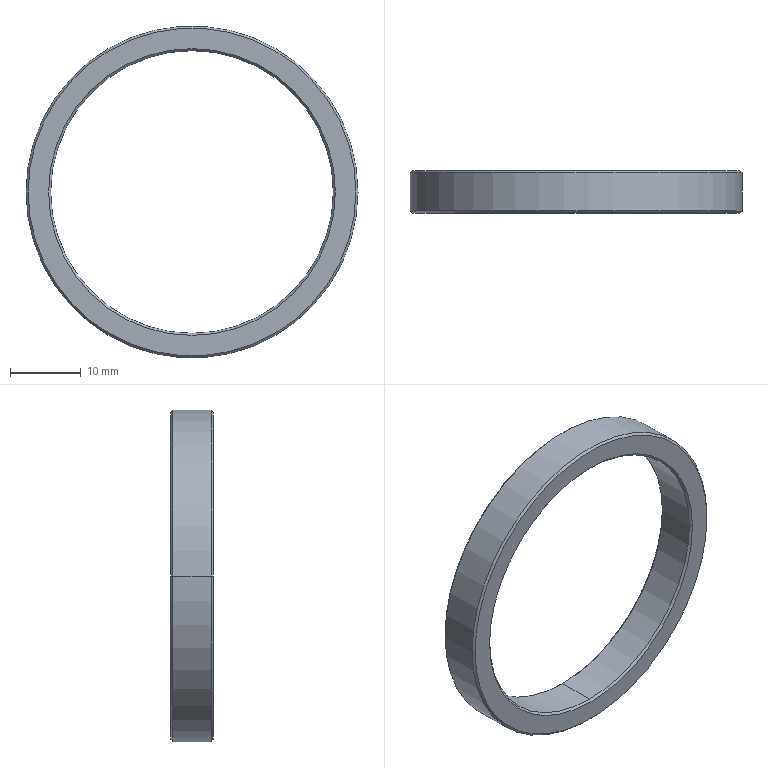Part | NX | 1 solid | 14 faces | box 47 x 6 x 47 mm | volume 2845 mm3 | cone 8 | cylinder 4 | plane 2 | commonest cylinder face diameters 40 x2 47 x2
STEP:
#1=CARTESIAN_POINT('',(23.2,0.,0.));
#2=VERTEX_POINT('',#1);
#3=CARTESIAN_POINT('',(-23.2,0.,0.));
#4=VERTEX_POINT('',#3);
#5=CARTESIAN_POINT('',(0.,0.,0.));
#6=DIRECTION('',(0.,1.,0.));
#7=DIRECTION('',(1.,0.,0.));
#8=AXIS2_PLACEMENT_3D('',#5,#6,#7);
#9=CIRCLE('',#8,23.2);
#10=EDGE_CURVE('',#2,#4,#9,.T.);
#11=ORIENTED_EDGE('',*,*,#10,.F.);
#12=CARTESIAN_POINT('',(0.,0.,0.));
#13=DIRECTION('',(0.,1.,0.));
#14=DIRECTION('',(1.,0.,0.));
#15=AXIS2_PLACEMENT_3D('',#12,#13,#14);
#16=CIRCLE('',#15,23.2);
#17=EDGE_CURVE('',#4,#2,#16,.T.);
#18=ORIENTED_EDGE('',*,*,#17,.F.);
#19=EDGE_LOOP('',(#11,#18));
#20=FACE_BOUND('',#19,.T.);
#21=CARTESIAN_POINT('',(20.3,0.,0.));
#22=VERTEX_POINT('',#21);
#23=CARTESIAN_POINT('',(-20.3,0.,0.));
#24=VERTEX_POINT('',#23);
#25=CARTESIAN_POINT('',(0.,0.,0.));
#26=DIRECTION('',(0.,-1.,0.));
#27=DIRECTION('',(-1.,0.,0.));
#28=AXIS2_PLACEMENT_3D('',#25,#26,#27);
#29=CIRCLE('',#28,20.3);
#30=EDGE_CURVE('',#22,#24,#29,.T.);
#31=ORIENTED_EDGE('',*,*,#30,.F.);
#32=CARTESIAN_POINT('',(0.,0.,0.));
#33=DIRECTION('',(0.,-1.,0.));
#34=DIRECTION('',(-1.,0.,0.));
#35=AXIS2_PLACEMENT_3D('',#32,#33,#34);
#36=CIRCLE('',#35,20.3);
#37=EDGE_CURVE('',#24,#22,#36,.T.);
#38=ORIENTED_EDGE('',*,*,#37,.F.);
#39=EDGE_LOOP('',(#31,#38));
#40=FACE_BOUND('',#39,.T.);
#41=CARTESIAN_POINT('',(0.,0.,0.));
#42=DIRECTION('',(0.,1.,0.));
#43=DIRECTION('',(1.,0.,0.));
#44=AXIS2_PLACEMENT_3D('',#41,#42,#43);
#45=PLANE('',#44);
#46=ADVANCED_FACE('',(#20,#40),#45,.F.);
#47=CARTESIAN_POINT('',(23.5,5.7,0.));
#48=VERTEX_POINT('',#47);
#49=CARTESIAN_POINT('',(-23.5,5.7,0.));
#50=VERTEX_POINT('',#49);
#51=CARTESIAN_POINT('',(0.,5.7,0.));
#52=DIRECTION('',(0.,-1.,0.));
#53=DIRECTION('',(-1.,0.,0.));
#54=AXIS2_PLACEMENT_3D('',#51,#52,#53);
#55=CIRCLE('',#54,23.5);
#56=EDGE_CURVE('',#48,#50,#55,.T.);
#57=ORIENTED_EDGE('',*,*,#56,.T.);
#58=CARTESIAN_POINT('',(-23.5,0.3,0.));
#59=VERTEX_POINT('',#58);
#60=CARTESIAN_POINT('',(-23.5,0.,0.));
#61=DIRECTION('',(0.,1.,0.));
#62=VECTOR('',#61,1000.);
#63=LINE('',#60,#62);
#64=EDGE_CURVE('',#50,#59,#63,.F.);
#65=ORIENTED_EDGE('',*,*,#64,.T.);
#66=CARTESIAN_POINT('',(23.5,0.3,0.));
#67=VERTEX_POINT('',#66);
#68=CARTESIAN_POINT('',(0.,0.3,0.));
#69=DIRECTION('',(0.,1.,0.));
#70=DIRECTION('',(1.,0.,0.));
#71=AXIS2_PLACEMENT_3D('',#68,#69,#70);
#72=CIRCLE('',#71,23.5);
#73=EDGE_CURVE('',#59,#67,#72,.T.);
#74=ORIENTED_EDGE('',*,*,#73,.T.);
#75=CARTESIAN_POINT('',(23.5,0.,0.));
#76=DIRECTION('',(0.,1.,0.));
#77=VECTOR('',#76,1000.);
#78=LINE('',#75,#77);
#79=EDGE_CURVE('',#48,#67,#78,.F.);
#80=ORIENTED_EDGE('',*,*,#79,.F.);
#81=EDGE_LOOP('',(#57,#65,#74,#80));
#82=FACE_BOUND('',#81,.T.);
#83=CARTESIAN_POINT('',(0.,0.,0.));
#84=DIRECTION('',(0.,1.,0.));
#85=DIRECTION('',(1.,0.,0.));
#86=AXIS2_PLACEMENT_3D('',#83,#84,#85);
#87=CYLINDRICAL_SURFACE('',#86,23.5);
#88=ADVANCED_FACE('',(#82),#87,.T.);
#89=CARTESIAN_POINT('',(0.,5.7,-20.));
#90=VERTEX_POINT('',#89);
#91=CARTESIAN_POINT('',(-20.,5.7,0.));
#92=VERTEX_POINT('',#91);
#93=CARTESIAN_POINT('',(0.,5.7,0.));
#94=DIRECTION('',(0.,1.,0.));
#95=DIRECTION('',(1.,0.,0.));
#96=AXIS2_PLACEMENT_3D('',#93,#94,#95);
#97=CIRCLE('',#96,20.);
#98=EDGE_CURVE('',#90,#92,#97,.T.);
#99=ORIENTED_EDGE('',*,*,#98,.T.);
#100=CARTESIAN_POINT('',(0.,5.7,20.));
#101=VERTEX_POINT('',#100);
#102=CARTESIAN_POINT('',(0.,5.7,0.));
#103=DIRECTION('',(0.,1.,0.));
#104=DIRECTION('',(1.,0.,0.));
#105=AXIS2_PLACEMENT_3D('',#102,#103,#104);
#106=CIRCLE('',#105,20.);
#107=EDGE_CURVE('',#92,#101,#106,.T.);
#108=ORIENTED_EDGE('',*,*,#107,.T.);
#109=CARTESIAN_POINT('',(0.,0.3,20.));
#110=VERTEX_POINT('',#109);
#111=CARTESIAN_POINT('',(0.,6.,20.));
#112=DIRECTION('',(0.,1.,0.));
#113=VECTOR('',#112,1000.);
#114=LINE('',#111,#113);
#115=EDGE_CURVE('',#110,#101,#114,.T.);
#116=ORIENTED_EDGE('',*,*,#115,.F.);
#117=CARTESIAN_POINT('',(-20.,0.3,0.));
#118=VERTEX_POINT('',#117);
#119=CARTESIAN_POINT('',(0.,0.3,0.));
#120=DIRECTION('',(0.,-1.,0.));
#121=DIRECTION('',(-1.,0.,0.));
#122=AXIS2_PLACEMENT_3D('',#119,#120,#121);
#123=CIRCLE('',#122,20.);
#124=EDGE_CURVE('',#110,#118,#123,.T.);
#125=ORIENTED_EDGE('',*,*,#124,.T.);
#126=CARTESIAN_POINT('',(0.,0.3,-20.));
#127=VERTEX_POINT('',#126);
#128=CARTESIAN_POINT('',(0.,0.3,0.));
#129=DIRECTION('',(0.,-1.,0.));
#130=DIRECTION('',(-1.,0.,0.));
#131=AXIS2_PLACEMENT_3D('',#128,#129,#130);
#132=CIRCLE('',#131,20.);
#133=EDGE_CURVE('',#118,#127,#132,.T.);
#134=ORIENTED_EDGE('',*,*,#133,.T.);
#135=CARTESIAN_POINT('',(0.,6.,-20.));
#136=DIRECTION('',(0.,1.,0.));
#137=VECTOR('',#136,1000.);
#138=LINE('',#135,#137);
#139=EDGE_CURVE('',#127,#90,#138,.T.);
#140=ORIENTED_EDGE('',*,*,#139,.T.);
#141=EDGE_LOOP('',(#99,#108,#116,#125,#134,#140));
#142=FACE_BOUND('',#141,.T.);
#143=CARTESIAN_POINT('',(0.,6.,0.));
#144=DIRECTION('',(0.,1.,0.));
#145=DIRECTION('',(0.,0.,-1.));
#146=AXIS2_PLACEMENT_3D('',#143,#144,#145);
#147=CYLINDRICAL_SURFACE('',#146,20.);
#148=ADVANCED_FACE('',(#142),#147,.F.);
#149=CARTESIAN_POINT('',(23.2,6.,0.));
#150=VERTEX_POINT('',#149);
#151=CARTESIAN_POINT('',(-23.2,6.,0.));
#152=VERTEX_POINT('',#151);
#153=CARTESIAN_POINT('',(0.,6.,0.));
#154=DIRECTION('',(0.,-1.,0.));
#155=DIRECTION('',(-1.,0.,0.));
#156=AXIS2_PLACEMENT_3D('',#153,#154,#155);
#157=CIRCLE('',#156,23.2);
#158=EDGE_CURVE('',#150,#152,#157,.T.);
#159=ORIENTED_EDGE('',*,*,#158,.F.);
#160=CARTESIAN_POINT('',(0.,6.,0.));
#161=DIRECTION('',(0.,-1.,0.));
#162=DIRECTION('',(-1.,0.,0.));
#163=AXIS2_PLACEMENT_3D('',#160,#161,#162);
#164=CIRCLE('',#163,23.2);
#165=EDGE_CURVE('',#152,#150,#164,.T.);
#166=ORIENTED_EDGE('',*,*,#165,.F.);
#167=EDGE_LOOP('',(#159,#166));
#168=FACE_BOUND('',#167,.T.);
#169=CARTESIAN_POINT('',(20.3,6.,0.));
#170=VERTEX_POINT('',#169);
#171=CARTESIAN_POINT('',(-20.3,6.,0.));
#172=VERTEX_POINT('',#171);
#173=CARTESIAN_POINT('',(0.,6.,0.));
#174=DIRECTION('',(0.,1.,0.));
#175=DIRECTION('',(1.,0.,0.));
#176=AXIS2_PLACEMENT_3D('',#173,#174,#175);
#177=CIRCLE('',#176,20.3);
#178=EDGE_CURVE('',#170,#172,#177,.T.);
#179=ORIENTED_EDGE('',*,*,#178,.F.);
#180=CARTESIAN_POINT('',(0.,6.,0.));
#181=DIRECTION('',(0.,1.,0.));
#182=DIRECTION('',(1.,0.,0.));
#183=AXIS2_PLACEMENT_3D('',#180,#181,#182);
#184=CIRCLE('',#183,20.3);
#185=EDGE_CURVE('',#172,#170,#184,.T.);
#186=ORIENTED_EDGE('',*,*,#185,.F.);
#187=EDGE_LOOP('',(#179,#186));
#188=FACE_BOUND('',#187,.T.);
#189=CARTESIAN_POINT('',(0.,6.,0.));
#190=DIRECTION('',(0.,1.,0.));
#191=DIRECTION('',(1.,0.,0.));
#192=AXIS2_PLACEMENT_3D('',#189,#190,#191);
#193=PLANE('',#192);
#194=ADVANCED_FACE('',(#168,#188),#193,.T.);
#195=CARTESIAN_POINT('',(0.,0.3,0.));
#196=DIRECTION('',(0.,1.,0.));
#197=DIRECTION('',(1.,0.,0.));
#198=AXIS2_PLACEMENT_3D('',#195,#196,#197);
#199=CIRCLE('',#198,23.5);
#200=EDGE_CURVE('',#67,#59,#199,.T.);
#201=ORIENTED_EDGE('',*,*,#200,.F.);
#202=CARTESIAN_POINT('',(23.2,0.,0.));
#203=DIRECTION('',(0.7071,0.7071,0.));
#204=VECTOR('',#203,1000.);
#205=LINE('',#202,#204);
#206=EDGE_CURVE('',#2,#67,#205,.T.);
#207=ORIENTED_EDGE('',*,*,#206,.F.);
#208=ORIENTED_EDGE('',*,*,#10,.T.);
#209=CARTESIAN_POINT('',(-23.2,0.,0.));
#210=DIRECTION('',(-0.7071,0.7071,0.));
#211=VECTOR('',#210,1000.);
#212=LINE('',#209,#211);
#213=EDGE_CURVE('',#4,#59,#212,.T.);
#214=ORIENTED_EDGE('',*,*,#213,.T.);
#215=EDGE_LOOP('',(#201,#207,#208,#214));
#216=FACE_BOUND('',#215,.T.);
#217=CARTESIAN_POINT('',(0.,0.,0.));
#218=DIRECTION('',(0.,1.,0.));
#219=DIRECTION('',(1.,0.,0.));
#220=AXIS2_PLACEMENT_3D('',#217,#218,#219);
#221=CONICAL_SURFACE('',#220,23.2,0.7854);
#222=ADVANCED_FACE('',(#216),#221,.T.);
#223=ORIENTED_EDGE('',*,*,#30,.T.);
#224=CARTESIAN_POINT('',(-20.3,0.,0.));
#225=DIRECTION('',(-0.7071,-0.7071,0.));
#226=VECTOR('',#225,1000.);
#227=LINE('',#224,#226);
#228=EDGE_CURVE('',#24,#118,#227,.F.);
#229=ORIENTED_EDGE('',*,*,#228,.T.);
#230=ORIENTED_EDGE('',*,*,#124,.F.);
#231=CARTESIAN_POINT('',(20.,0.3,0.));
#232=VERTEX_POINT('',#231);
#233=CARTESIAN_POINT('',(0.,0.3,0.));
#234=DIRECTION('',(0.,-1.,0.));
#235=DIRECTION('',(-1.,0.,0.));
#236=AXIS2_PLACEMENT_3D('',#233,#234,#235);
#237=CIRCLE('',#236,20.);
#238=EDGE_CURVE('',#232,#110,#237,.T.);
#239=ORIENTED_EDGE('',*,*,#238,.F.);
#240=CARTESIAN_POINT('',(20.3,0.,0.));
#241=DIRECTION('',(0.7071,-0.7071,0.));
#242=VECTOR('',#241,1000.);
#243=LINE('',#240,#242);
#244=EDGE_CURVE('',#22,#232,#243,.F.);
#245=ORIENTED_EDGE('',*,*,#244,.F.);
#246=EDGE_LOOP('',(#223,#229,#230,#239,#245));
#247=FACE_BOUND('',#246,.T.);
#248=CARTESIAN_POINT('',(0.,0.,0.));
#249=DIRECTION('',(0.,-1.,0.));
#250=DIRECTION('',(-1.,0.,0.));
#251=AXIS2_PLACEMENT_3D('',#248,#249,#250);
#252=CONICAL_SURFACE('',#251,20.3,0.7854);
#253=ADVANCED_FACE('',(#247),#252,.F.);
#254=ORIENTED_EDGE('',*,*,#158,.T.);
#255=CARTESIAN_POINT('',(-23.5,5.7,0.));
#256=DIRECTION('',(-0.7071,-0.7071,0.));
#257=VECTOR('',#256,1000.);
#258=LINE('',#255,#257);
#259=EDGE_CURVE('',#50,#152,#258,.F.);
#260=ORIENTED_EDGE('',*,*,#259,.F.);
#261=ORIENTED_EDGE('',*,*,#56,.F.);
#262=CARTESIAN_POINT('',(23.5,5.7,0.));
#263=DIRECTION('',(0.7071,-0.7071,0.));
#264=VECTOR('',#263,1000.);
#265=LINE('',#262,#264);
#266=EDGE_CURVE('',#48,#150,#265,.F.);
#267=ORIENTED_EDGE('',*,*,#266,.T.);
#268=EDGE_LOOP('',(#254,#260,#261,#267));
#269=FACE_BOUND('',#268,.T.);
#270=CARTESIAN_POINT('',(0.,5.7,0.));
#271=DIRECTION('',(0.,-1.,0.));
#272=DIRECTION('',(-1.,0.,0.));
#273=AXIS2_PLACEMENT_3D('',#270,#271,#272);
#274=CONICAL_SURFACE('',#273,23.5,0.7854);
#275=ADVANCED_FACE('',(#269),#274,.T.);
#276=ORIENTED_EDGE('',*,*,#98,.F.);
#277=CARTESIAN_POINT('',(20.,5.7,0.));
#278=VERTEX_POINT('',#277);
#279=CARTESIAN_POINT('',(0.,5.7,0.));
#280=DIRECTION('',(0.,1.,0.));
#281=DIRECTION('',(1.,0.,0.));
#282=AXIS2_PLACEMENT_3D('',#279,#280,#281);
#283=CIRCLE('',#282,20.);
#284=EDGE_CURVE('',#278,#90,#283,.T.);
#285=ORIENTED_EDGE('',*,*,#284,.F.);
#286=CARTESIAN_POINT('',(20.3,6.,0.));
#287=DIRECTION('',(0.7071,0.7071,0.));
#288=VECTOR('',#287,1000.);
#289=LINE('',#286,#288);
#290=EDGE_CURVE('',#278,#170,#289,.T.);
#291=ORIENTED_EDGE('',*,*,#290,.T.);
#292=ORIENTED_EDGE('',*,*,#178,.T.);
#293=CARTESIAN_POINT('',(-20.3,6.,0.));
#294=DIRECTION('',(-0.7071,0.7071,0.));
#295=VECTOR('',#294,1000.);
#296=LINE('',#293,#295);
#297=EDGE_CURVE('',#92,#172,#296,.T.);
#298=ORIENTED_EDGE('',*,*,#297,.F.);
#299=EDGE_LOOP('',(#276,#285,#291,#292,#298));
#300=FACE_BOUND('',#299,.T.);
#301=CARTESIAN_POINT('',(0.,6.,0.));
#302=DIRECTION('',(0.,1.,0.));
#303=DIRECTION('',(1.,0.,0.));
#304=AXIS2_PLACEMENT_3D('',#301,#302,#303);
#305=CONICAL_SURFACE('',#304,20.3,0.7854);
#306=ADVANCED_FACE('',(#300),#305,.F.);
#307=CARTESIAN_POINT('',(0.,0.3,0.));
#308=DIRECTION('',(0.,-1.,0.));
#309=DIRECTION('',(-1.,0.,0.));
#310=AXIS2_PLACEMENT_3D('',#307,#308,#309);
#311=CIRCLE('',#310,20.);
#312=EDGE_CURVE('',#127,#232,#311,.T.);
#313=ORIENTED_EDGE('',*,*,#312,.T.);
#314=ORIENTED_EDGE('',*,*,#238,.T.);
#315=ORIENTED_EDGE('',*,*,#115,.T.);
#316=CARTESIAN_POINT('',(0.,5.7,0.));
#317=DIRECTION('',(0.,1.,0.));
#318=DIRECTION('',(1.,0.,0.));
#319=AXIS2_PLACEMENT_3D('',#316,#317,#318);
#320=CIRCLE('',#319,20.);
#321=EDGE_CURVE('',#101,#278,#320,.T.);
#322=ORIENTED_EDGE('',*,*,#321,.T.);
#323=ORIENTED_EDGE('',*,*,#284,.T.);
#324=ORIENTED_EDGE('',*,*,#139,.F.);
#325=EDGE_LOOP('',(#313,#314,#315,#322,#323,#324));
#326=FACE_BOUND('',#325,.T.);
#327=CARTESIAN_POINT('',(0.,6.,0.));
#328=DIRECTION('',(0.,1.,0.));
#329=DIRECTION('',(0.,0.,-1.));
#330=AXIS2_PLACEMENT_3D('',#327,#328,#329);
#331=CYLINDRICAL_SURFACE('',#330,20.);
#332=ADVANCED_FACE('',(#326),#331,.F.);
#333=ORIENTED_EDGE('',*,*,#290,.F.);
#334=ORIENTED_EDGE('',*,*,#321,.F.);
#335=ORIENTED_EDGE('',*,*,#107,.F.);
#336=ORIENTED_EDGE('',*,*,#297,.T.);
#337=ORIENTED_EDGE('',*,*,#185,.T.);
#338=EDGE_LOOP('',(#333,#334,#335,#336,#337));
#339=FACE_BOUND('',#338,.T.);
#340=CARTESIAN_POINT('',(0.,6.,0.));
#341=DIRECTION('',(0.,1.,0.));
#342=DIRECTION('',(1.,0.,0.));
#343=AXIS2_PLACEMENT_3D('',#340,#341,#342);
#344=CONICAL_SURFACE('',#343,20.3,0.7854);
#345=ADVANCED_FACE('',(#339),#344,.F.);
#346=ORIENTED_EDGE('',*,*,#259,.T.);
#347=ORIENTED_EDGE('',*,*,#165,.T.);
#348=ORIENTED_EDGE('',*,*,#266,.F.);
#349=CARTESIAN_POINT('',(0.,5.7,0.));
#350=DIRECTION('',(0.,-1.,0.));
#351=DIRECTION('',(-1.,0.,0.));
#352=AXIS2_PLACEMENT_3D('',#349,#350,#351);
#353=CIRCLE('',#352,23.5);
#354=EDGE_CURVE('',#50,#48,#353,.T.);
#355=ORIENTED_EDGE('',*,*,#354,.F.);
#356=EDGE_LOOP('',(#346,#347,#348,#355));
#357=FACE_BOUND('',#356,.T.);
#358=CARTESIAN_POINT('',(0.,5.7,0.));
#359=DIRECTION('',(0.,-1.,0.));
#360=DIRECTION('',(-1.,0.,0.));
#361=AXIS2_PLACEMENT_3D('',#358,#359,#360);
#362=CONICAL_SURFACE('',#361,23.5,0.7854);
#363=ADVANCED_FACE('',(#357),#362,.T.);
#364=ORIENTED_EDGE('',*,*,#200,.T.);
#365=ORIENTED_EDGE('',*,*,#64,.F.);
#366=ORIENTED_EDGE('',*,*,#354,.T.);
#367=ORIENTED_EDGE('',*,*,#79,.T.);
#368=EDGE_LOOP('',(#364,#365,#366,#367));
#369=FACE_BOUND('',#368,.T.);
#370=CARTESIAN_POINT('',(0.,0.,0.));
#371=DIRECTION('',(0.,1.,0.));
#372=DIRECTION('',(1.,0.,0.));
#373=AXIS2_PLACEMENT_3D('',#370,#371,#372);
#374=CYLINDRICAL_SURFACE('',#373,23.5);
#375=ADVANCED_FACE('',(#369),#374,.T.);
#376=ORIENTED_EDGE('',*,*,#206,.T.);
#377=ORIENTED_EDGE('',*,*,#73,.F.);
#378=ORIENTED_EDGE('',*,*,#213,.F.);
#379=ORIENTED_EDGE('',*,*,#17,.T.);
#380=EDGE_LOOP('',(#376,#377,#378,#379));
#381=FACE_BOUND('',#380,.T.);
#382=CARTESIAN_POINT('',(0.,0.,0.));
#383=DIRECTION('',(0.,1.,0.));
#384=DIRECTION('',(1.,0.,0.));
#385=AXIS2_PLACEMENT_3D('',#382,#383,#384);
#386=CONICAL_SURFACE('',#385,23.2,0.7854);
#387=ADVANCED_FACE('',(#381),#386,.T.);
#388=ORIENTED_EDGE('',*,*,#312,.F.);
#389=ORIENTED_EDGE('',*,*,#133,.F.);
#390=ORIENTED_EDGE('',*,*,#228,.F.);
#391=ORIENTED_EDGE('',*,*,#37,.T.);
#392=ORIENTED_EDGE('',*,*,#244,.T.);
#393=EDGE_LOOP('',(#388,#389,#390,#391,#392));
#394=FACE_BOUND('',#393,.T.);
#395=CARTESIAN_POINT('',(0.,0.,0.));
#396=DIRECTION('',(0.,-1.,0.));
#397=DIRECTION('',(-1.,0.,0.));
#398=AXIS2_PLACEMENT_3D('',#395,#396,#397);
#399=CONICAL_SURFACE('',#398,20.3,0.7854);
#400=ADVANCED_FACE('',(#394),#399,.F.);
#401=CLOSED_SHELL('',(#46,#88,#148,#194,#222,#253,#275,#306,#332,#345,#363,#375,#387,#400));
#402=MANIFOLD_SOLID_BREP('',#401);
#403=(LENGTH_UNIT()NAMED_UNIT(*)SI_UNIT(.MILLI.,.METRE.));
#404=UNCERTAINTY_MEASURE_WITH_UNIT(LENGTH_MEASURE(0.00001),#403,'','');
#405=(NAMED_UNIT(*)PLANE_ANGLE_UNIT()SI_UNIT($,.RADIAN.));
#406=(NAMED_UNIT(*)SI_UNIT($,.STERADIAN.)SOLID_ANGLE_UNIT());
#407=(GEOMETRIC_REPRESENTATION_CONTEXT(3)GLOBAL_UNCERTAINTY_ASSIGNED_CONTEXT((#404))GLOBAL_UNIT_ASSIGNED_CONTEXT((#403,#405,#406))REPRESENTATION_CONTEXT('',''));
#408=ADVANCED_BREP_SHAPE_REPRESENTATION('',(#402),#407);